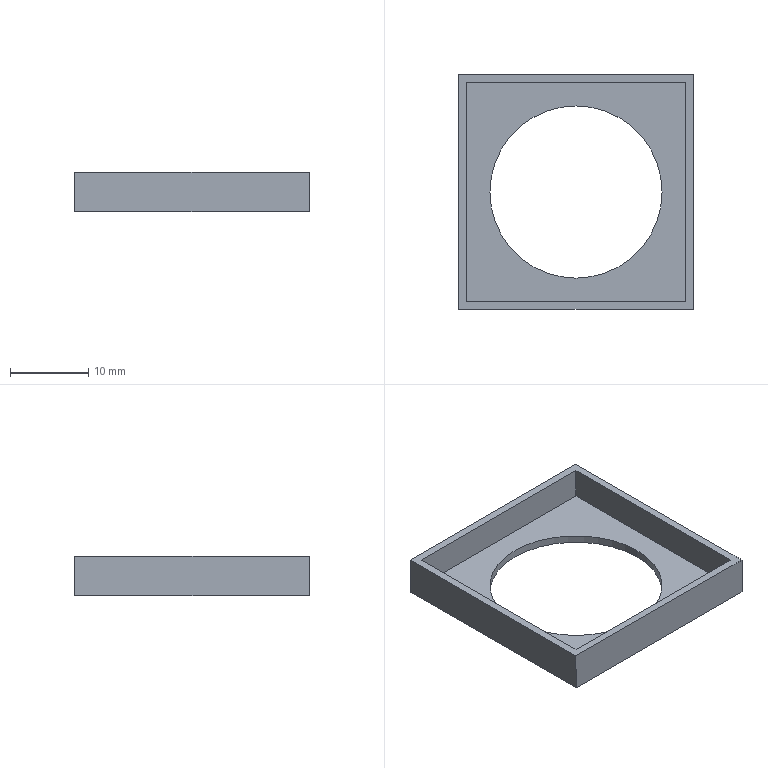Part | SolidWorks | features BossThin 1, Extrusion 1, ICE 1 | 1 solid | 13 faces | box 30 x 30 x 5 mm | volume 983.867 mm3 | plane 11 | cylinder 2 | commonest cylinder face diameters 22 x2
STEP:
#1=CARTESIAN_POINT('',(-11.,0.,0.));
#2=VERTEX_POINT('',#1);
#3=CARTESIAN_POINT('',(11.,0.,0.));
#4=VERTEX_POINT('',#3);
#5=CARTESIAN_POINT('',(0.,0.,0.));
#6=DIRECTION('',(0.,0.,1.));
#7=DIRECTION('',(1.,0.,0.));
#8=AXIS2_PLACEMENT_3D('',#5,#6,#7);
#9=CIRCLE('',#8,11.);
#10=EDGE_CURVE('',#2,#4,#9,.T.);
#11=ORIENTED_EDGE('',*,*,#10,.F.);
#12=CARTESIAN_POINT('',(-11.,0.,1.));
#13=VERTEX_POINT('',#12);
#14=CARTESIAN_POINT('',(-11.,0.,-4.));
#15=DIRECTION('',(0.,0.,1.));
#16=VECTOR('',#15,1000.);
#17=LINE('',#14,#16);
#18=EDGE_CURVE('',#2,#13,#17,.T.);
#19=ORIENTED_EDGE('',*,*,#18,.T.);
#20=CARTESIAN_POINT('',(11.,0.,1.));
#21=VERTEX_POINT('',#20);
#22=CARTESIAN_POINT('',(0.,0.,1.));
#23=DIRECTION('',(0.,0.,1.));
#24=DIRECTION('',(1.,0.,0.));
#25=AXIS2_PLACEMENT_3D('',#22,#23,#24);
#26=CIRCLE('',#25,11.);
#27=EDGE_CURVE('',#13,#21,#26,.T.);
#28=ORIENTED_EDGE('',*,*,#27,.T.);
#29=CARTESIAN_POINT('',(11.,0.,-4.));
#30=DIRECTION('',(0.,0.,1.));
#31=VECTOR('',#30,1000.);
#32=LINE('',#29,#31);
#33=EDGE_CURVE('',#4,#21,#32,.T.);
#34=ORIENTED_EDGE('',*,*,#33,.F.);
#35=EDGE_LOOP('',(#11,#19,#28,#34));
#36=FACE_OUTER_BOUND('',#35,.T.);
#37=CARTESIAN_POINT('',(0.,0.,-4.));
#38=DIRECTION('',(0.,0.,1.));
#39=DIRECTION('',(1.,0.,0.));
#40=AXIS2_PLACEMENT_3D('',#37,#38,#39);
#41=CYLINDRICAL_SURFACE('',#40,11.);
#42=ADVANCED_FACE('',(#36),#41,.F.);
#43=CARTESIAN_POINT('',(0.,0.,1.));
#44=DIRECTION('',(0.,0.,1.));
#45=DIRECTION('',(1.,0.,0.));
#46=AXIS2_PLACEMENT_3D('',#43,#44,#45);
#47=CIRCLE('',#46,11.);
#48=EDGE_CURVE('',#21,#13,#47,.T.);
#49=ORIENTED_EDGE('',*,*,#48,.F.);
#50=ORIENTED_EDGE('',*,*,#27,.F.);
#51=EDGE_LOOP('',(#49,#50));
#52=FACE_BOUND('',#51,.T.);
#53=CARTESIAN_POINT('',(14.,-14.,1.));
#54=VERTEX_POINT('',#53);
#55=CARTESIAN_POINT('',(14.,14.,1.));
#56=VERTEX_POINT('',#55);
#57=CARTESIAN_POINT('',(14.,14.,1.));
#58=DIRECTION('',(0.,1.,0.));
#59=VECTOR('',#58,1000.);
#60=LINE('',#57,#59);
#61=EDGE_CURVE('',#54,#56,#60,.T.);
#62=ORIENTED_EDGE('',*,*,#61,.T.);
#63=CARTESIAN_POINT('',(-14.,14.,1.));
#64=VERTEX_POINT('',#63);
#65=CARTESIAN_POINT('',(-14.,14.,1.));
#66=DIRECTION('',(-1.,0.,0.));
#67=VECTOR('',#66,1000.);
#68=LINE('',#65,#67);
#69=EDGE_CURVE('',#56,#64,#68,.T.);
#70=ORIENTED_EDGE('',*,*,#69,.T.);
#71=CARTESIAN_POINT('',(-14.,-14.,1.));
#72=VERTEX_POINT('',#71);
#73=CARTESIAN_POINT('',(-14.,14.,1.));
#74=DIRECTION('',(0.,-1.,0.));
#75=VECTOR('',#74,1000.);
#76=LINE('',#73,#75);
#77=EDGE_CURVE('',#64,#72,#76,.T.);
#78=ORIENTED_EDGE('',*,*,#77,.T.);
#79=CARTESIAN_POINT('',(-14.,-14.,1.));
#80=DIRECTION('',(1.,0.,0.));
#81=VECTOR('',#80,1000.);
#82=LINE('',#79,#81);
#83=EDGE_CURVE('',#72,#54,#82,.T.);
#84=ORIENTED_EDGE('',*,*,#83,.T.);
#85=EDGE_LOOP('',(#62,#70,#78,#84));
#86=FACE_OUTER_BOUND('',#85,.T.);
#87=CARTESIAN_POINT('',(0.,0.,1.));
#88=DIRECTION('',(0.,0.,1.));
#89=DIRECTION('',(1.,0.,0.));
#90=AXIS2_PLACEMENT_3D('',#87,#88,#89);
#91=PLANE('',#90);
#92=ADVANCED_FACE('',(#52,#86),#91,.T.);
#93=CARTESIAN_POINT('',(15.,-15.,5.));
#94=VERTEX_POINT('',#93);
#95=CARTESIAN_POINT('',(15.,15.,5.));
#96=VERTEX_POINT('',#95);
#97=CARTESIAN_POINT('',(15.,14.,5.));
#98=DIRECTION('',(0.,1.,0.));
#99=VECTOR('',#98,1000.);
#100=LINE('',#97,#99);
#101=EDGE_CURVE('',#94,#96,#100,.T.);
#102=ORIENTED_EDGE('',*,*,#101,.T.);
#103=CARTESIAN_POINT('',(-15.,15.,5.));
#104=VERTEX_POINT('',#103);
#105=CARTESIAN_POINT('',(-14.,15.,5.));
#106=DIRECTION('',(-1.,0.,0.));
#107=VECTOR('',#106,1000.);
#108=LINE('',#105,#107);
#109=EDGE_CURVE('',#96,#104,#108,.T.);
#110=ORIENTED_EDGE('',*,*,#109,.T.);
#111=CARTESIAN_POINT('',(-15.,-15.,5.));
#112=VERTEX_POINT('',#111);
#113=CARTESIAN_POINT('',(-15.,14.,5.));
#114=DIRECTION('',(0.,-1.,0.));
#115=VECTOR('',#114,1000.);
#116=LINE('',#113,#115);
#117=EDGE_CURVE('',#104,#112,#116,.T.);
#118=ORIENTED_EDGE('',*,*,#117,.T.);
#119=CARTESIAN_POINT('',(-14.,-15.,5.));
#120=DIRECTION('',(1.,0.,0.));
#121=VECTOR('',#120,1000.);
#122=LINE('',#119,#121);
#123=EDGE_CURVE('',#112,#94,#122,.T.);
#124=ORIENTED_EDGE('',*,*,#123,.T.);
#125=EDGE_LOOP('',(#102,#110,#118,#124));
#126=FACE_OUTER_BOUND('',#125,.T.);
#127=CARTESIAN_POINT('',(14.,14.,5.));
#128=VERTEX_POINT('',#127);
#129=CARTESIAN_POINT('',(-14.,14.,5.));
#130=VERTEX_POINT('',#129);
#131=CARTESIAN_POINT('',(-14.,14.,5.));
#132=DIRECTION('',(-1.,0.,0.));
#133=VECTOR('',#132,1000.);
#134=LINE('',#131,#133);
#135=EDGE_CURVE('',#128,#130,#134,.T.);
#136=ORIENTED_EDGE('',*,*,#135,.F.);
#137=CARTESIAN_POINT('',(14.,-14.,5.));
#138=VERTEX_POINT('',#137);
#139=CARTESIAN_POINT('',(14.,14.,5.));
#140=DIRECTION('',(0.,1.,0.));
#141=VECTOR('',#140,1000.);
#142=LINE('',#139,#141);
#143=EDGE_CURVE('',#138,#128,#142,.T.);
#144=ORIENTED_EDGE('',*,*,#143,.F.);
#145=CARTESIAN_POINT('',(-14.,-14.,5.));
#146=VERTEX_POINT('',#145);
#147=CARTESIAN_POINT('',(-14.,-14.,5.));
#148=DIRECTION('',(1.,0.,0.));
#149=VECTOR('',#148,1000.);
#150=LINE('',#147,#149);
#151=EDGE_CURVE('',#146,#138,#150,.T.);
#152=ORIENTED_EDGE('',*,*,#151,.F.);
#153=CARTESIAN_POINT('',(-14.,14.,5.));
#154=DIRECTION('',(0.,-1.,0.));
#155=VECTOR('',#154,1000.);
#156=LINE('',#153,#155);
#157=EDGE_CURVE('',#130,#146,#156,.T.);
#158=ORIENTED_EDGE('',*,*,#157,.F.);
#159=EDGE_LOOP('',(#136,#144,#152,#158));
#160=FACE_BOUND('',#159,.T.);
#161=CARTESIAN_POINT('',(0.,0.,5.));
#162=DIRECTION('',(0.,0.,1.));
#163=DIRECTION('',(1.,0.,0.));
#164=AXIS2_PLACEMENT_3D('',#161,#162,#163);
#165=PLANE('',#164);
#166=ADVANCED_FACE('',(#126,#160),#165,.T.);
#167=CARTESIAN_POINT('',(15.,-15.,0.));
#168=VERTEX_POINT('',#167);
#169=CARTESIAN_POINT('',(15.,15.,0.));
#170=VERTEX_POINT('',#169);
#171=CARTESIAN_POINT('',(15.,14.,0.));
#172=DIRECTION('',(0.,1.,0.));
#173=VECTOR('',#172,1000.);
#174=LINE('',#171,#173);
#175=EDGE_CURVE('',#168,#170,#174,.T.);
#176=ORIENTED_EDGE('',*,*,#175,.T.);
#177=CARTESIAN_POINT('',(15.,15.,5.));
#178=DIRECTION('',(0.,0.,-1.));
#179=VECTOR('',#178,1000.);
#180=LINE('',#177,#179);
#181=EDGE_CURVE('',#96,#170,#180,.T.);
#182=ORIENTED_EDGE('',*,*,#181,.F.);
#183=ORIENTED_EDGE('',*,*,#101,.F.);
#184=CARTESIAN_POINT('',(15.,-15.,5.));
#185=DIRECTION('',(0.,0.,-1.));
#186=VECTOR('',#185,1000.);
#187=LINE('',#184,#186);
#188=EDGE_CURVE('',#94,#168,#187,.T.);
#189=ORIENTED_EDGE('',*,*,#188,.T.);
#190=EDGE_LOOP('',(#176,#182,#183,#189));
#191=FACE_OUTER_BOUND('',#190,.T.);
#192=CARTESIAN_POINT('',(15.,14.,5.));
#193=DIRECTION('',(-1.,0.,0.));
#194=DIRECTION('',(0.,-1.,0.));
#195=AXIS2_PLACEMENT_3D('',#192,#193,#194);
#196=PLANE('',#195);
#197=ADVANCED_FACE('',(#191),#196,.F.);
#198=CARTESIAN_POINT('',(-15.,15.,0.));
#199=VERTEX_POINT('',#198);
#200=CARTESIAN_POINT('',(-14.,15.,0.));
#201=DIRECTION('',(-1.,0.,0.));
#202=VECTOR('',#201,1000.);
#203=LINE('',#200,#202);
#204=EDGE_CURVE('',#170,#199,#203,.T.);
#205=ORIENTED_EDGE('',*,*,#204,.T.);
#206=CARTESIAN_POINT('',(-15.,15.,5.));
#207=DIRECTION('',(0.,0.,-1.));
#208=VECTOR('',#207,1000.);
#209=LINE('',#206,#208);
#210=EDGE_CURVE('',#104,#199,#209,.T.);
#211=ORIENTED_EDGE('',*,*,#210,.F.);
#212=ORIENTED_EDGE('',*,*,#109,.F.);
#213=ORIENTED_EDGE('',*,*,#181,.T.);
#214=EDGE_LOOP('',(#205,#211,#212,#213));
#215=FACE_OUTER_BOUND('',#214,.T.);
#216=CARTESIAN_POINT('',(-14.,15.,5.));
#217=DIRECTION('',(0.,-1.,0.));
#218=DIRECTION('',(0.,0.,-1.));
#219=AXIS2_PLACEMENT_3D('',#216,#217,#218);
#220=PLANE('',#219);
#221=ADVANCED_FACE('',(#215),#220,.F.);
#222=CARTESIAN_POINT('',(-15.,-15.,0.));
#223=VERTEX_POINT('',#222);
#224=CARTESIAN_POINT('',(-15.,14.,0.));
#225=DIRECTION('',(0.,-1.,0.));
#226=VECTOR('',#225,1000.);
#227=LINE('',#224,#226);
#228=EDGE_CURVE('',#199,#223,#227,.T.);
#229=ORIENTED_EDGE('',*,*,#228,.T.);
#230=CARTESIAN_POINT('',(-15.,-15.,5.));
#231=DIRECTION('',(0.,0.,-1.));
#232=VECTOR('',#231,1000.);
#233=LINE('',#230,#232);
#234=EDGE_CURVE('',#112,#223,#233,.T.);
#235=ORIENTED_EDGE('',*,*,#234,.F.);
#236=ORIENTED_EDGE('',*,*,#117,.F.);
#237=ORIENTED_EDGE('',*,*,#210,.T.);
#238=EDGE_LOOP('',(#229,#235,#236,#237));
#239=FACE_OUTER_BOUND('',#238,.T.);
#240=CARTESIAN_POINT('',(-15.,14.,5.));
#241=DIRECTION('',(1.,0.,0.));
#242=DIRECTION('',(0.,1.,0.));
#243=AXIS2_PLACEMENT_3D('',#240,#241,#242);
#244=PLANE('',#243);
#245=ADVANCED_FACE('',(#239),#244,.F.);
#246=CARTESIAN_POINT('',(-14.,-15.,0.));
#247=DIRECTION('',(1.,0.,0.));
#248=VECTOR('',#247,1000.);
#249=LINE('',#246,#248);
#250=EDGE_CURVE('',#223,#168,#249,.T.);
#251=ORIENTED_EDGE('',*,*,#250,.T.);
#252=ORIENTED_EDGE('',*,*,#188,.F.);
#253=ORIENTED_EDGE('',*,*,#123,.F.);
#254=ORIENTED_EDGE('',*,*,#234,.T.);
#255=EDGE_LOOP('',(#251,#252,#253,#254));
#256=FACE_OUTER_BOUND('',#255,.T.);
#257=CARTESIAN_POINT('',(-14.,-15.,5.));
#258=DIRECTION('',(0.,1.,0.));
#259=DIRECTION('',(0.,0.,1.));
#260=AXIS2_PLACEMENT_3D('',#257,#258,#259);
#261=PLANE('',#260);
#262=ADVANCED_FACE('',(#256),#261,.F.);
#263=CARTESIAN_POINT('',(14.,14.,5.));
#264=DIRECTION('',(0.,0.,-1.));
#265=VECTOR('',#264,1000.);
#266=LINE('',#263,#265);
#267=EDGE_CURVE('',#128,#56,#266,.T.);
#268=ORIENTED_EDGE('',*,*,#267,.T.);
#269=ORIENTED_EDGE('',*,*,#61,.F.);
#270=CARTESIAN_POINT('',(14.,-14.,5.));
#271=DIRECTION('',(0.,0.,-1.));
#272=VECTOR('',#271,1000.);
#273=LINE('',#270,#272);
#274=EDGE_CURVE('',#138,#54,#273,.T.);
#275=ORIENTED_EDGE('',*,*,#274,.F.);
#276=ORIENTED_EDGE('',*,*,#143,.T.);
#277=EDGE_LOOP('',(#268,#269,#275,#276));
#278=FACE_OUTER_BOUND('',#277,.T.);
#279=CARTESIAN_POINT('',(14.,14.,5.));
#280=DIRECTION('',(-1.,0.,0.));
#281=DIRECTION('',(0.,-1.,0.));
#282=AXIS2_PLACEMENT_3D('',#279,#280,#281);
#283=PLANE('',#282);
#284=ADVANCED_FACE('',(#278),#283,.T.);
#285=CARTESIAN_POINT('',(-14.,14.,5.));
#286=DIRECTION('',(0.,0.,-1.));
#287=VECTOR('',#286,1000.);
#288=LINE('',#285,#287);
#289=EDGE_CURVE('',#130,#64,#288,.T.);
#290=ORIENTED_EDGE('',*,*,#289,.T.);
#291=ORIENTED_EDGE('',*,*,#69,.F.);
#292=ORIENTED_EDGE('',*,*,#267,.F.);
#293=ORIENTED_EDGE('',*,*,#135,.T.);
#294=EDGE_LOOP('',(#290,#291,#292,#293));
#295=FACE_OUTER_BOUND('',#294,.T.);
#296=CARTESIAN_POINT('',(-14.,14.,5.));
#297=DIRECTION('',(0.,-1.,0.));
#298=DIRECTION('',(0.,0.,-1.));
#299=AXIS2_PLACEMENT_3D('',#296,#297,#298);
#300=PLANE('',#299);
#301=ADVANCED_FACE('',(#295),#300,.T.);
#302=CARTESIAN_POINT('',(-14.,-14.,5.));
#303=DIRECTION('',(0.,0.,-1.));
#304=VECTOR('',#303,1000.);
#305=LINE('',#302,#304);
#306=EDGE_CURVE('',#146,#72,#305,.T.);
#307=ORIENTED_EDGE('',*,*,#306,.T.);
#308=ORIENTED_EDGE('',*,*,#77,.F.);
#309=ORIENTED_EDGE('',*,*,#289,.F.);
#310=ORIENTED_EDGE('',*,*,#157,.T.);
#311=EDGE_LOOP('',(#307,#308,#309,#310));
#312=FACE_OUTER_BOUND('',#311,.T.);
#313=CARTESIAN_POINT('',(-14.,14.,5.));
#314=DIRECTION('',(1.,0.,0.));
#315=DIRECTION('',(0.,1.,0.));
#316=AXIS2_PLACEMENT_3D('',#313,#314,#315);
#317=PLANE('',#316);
#318=ADVANCED_FACE('',(#312),#317,.T.);
#319=ORIENTED_EDGE('',*,*,#274,.T.);
#320=ORIENTED_EDGE('',*,*,#83,.F.);
#321=ORIENTED_EDGE('',*,*,#306,.F.);
#322=ORIENTED_EDGE('',*,*,#151,.T.);
#323=EDGE_LOOP('',(#319,#320,#321,#322));
#324=FACE_OUTER_BOUND('',#323,.T.);
#325=CARTESIAN_POINT('',(-14.,-14.,5.));
#326=DIRECTION('',(0.,1.,0.));
#327=DIRECTION('',(0.,0.,1.));
#328=AXIS2_PLACEMENT_3D('',#325,#326,#327);
#329=PLANE('',#328);
#330=ADVANCED_FACE('',(#324),#329,.T.);
#331=CARTESIAN_POINT('',(0.,0.,0.));
#332=DIRECTION('',(0.,0.,1.));
#333=DIRECTION('',(1.,0.,0.));
#334=AXIS2_PLACEMENT_3D('',#331,#332,#333);
#335=CIRCLE('',#334,11.);
#336=EDGE_CURVE('',#4,#2,#335,.T.);
#337=ORIENTED_EDGE('',*,*,#336,.T.);
#338=ORIENTED_EDGE('',*,*,#10,.T.);
#339=EDGE_LOOP('',(#337,#338));
#340=FACE_BOUND('',#339,.T.);
#341=ORIENTED_EDGE('',*,*,#175,.F.);
#342=ORIENTED_EDGE('',*,*,#250,.F.);
#343=ORIENTED_EDGE('',*,*,#228,.F.);
#344=ORIENTED_EDGE('',*,*,#204,.F.);
#345=EDGE_LOOP('',(#341,#342,#343,#344));
#346=FACE_OUTER_BOUND('',#345,.T.);
#347=CARTESIAN_POINT('',(0.,0.,0.));
#348=DIRECTION('',(0.,0.,1.));
#349=DIRECTION('',(1.,0.,0.));
#350=AXIS2_PLACEMENT_3D('',#347,#348,#349);
#351=PLANE('',#350);
#352=ADVANCED_FACE('',(#340,#346),#351,.F.);
#353=ORIENTED_EDGE('',*,*,#18,.F.);
#354=ORIENTED_EDGE('',*,*,#336,.F.);
#355=ORIENTED_EDGE('',*,*,#33,.T.);
#356=ORIENTED_EDGE('',*,*,#48,.T.);
#357=EDGE_LOOP('',(#353,#354,#355,#356));
#358=FACE_OUTER_BOUND('',#357,.T.);
#359=CARTESIAN_POINT('',(0.,0.,-4.));
#360=DIRECTION('',(0.,0.,1.));
#361=DIRECTION('',(1.,0.,0.));
#362=AXIS2_PLACEMENT_3D('',#359,#360,#361);
#363=CYLINDRICAL_SURFACE('',#362,11.);
#364=ADVANCED_FACE('',(#358),#363,.F.);
#365=CLOSED_SHELL('',(#42,#92,#166,#197,#221,#245,#262,#284,#301,#318,#330,#352,#364));
#366=MANIFOLD_SOLID_BREP('',#365);
#367=CARTESIAN_POINT('',(0.,0.,0.));
#368=DIRECTION('',(0.,0.,1.));
#369=DIRECTION('',(1.,0.,0.));
#370=AXIS2_PLACEMENT_3D('',#367,#368,#369);
#371=(LENGTH_UNIT()NAMED_UNIT(*)SI_UNIT(.MILLI.,.METRE.));
#372=UNCERTAINTY_MEASURE_WITH_UNIT(LENGTH_MEASURE(0.00001),#371,'','');
#373=(NAMED_UNIT(*)PLANE_ANGLE_UNIT()SI_UNIT($,.RADIAN.));
#374=(NAMED_UNIT(*)SI_UNIT($,.STERADIAN.)SOLID_ANGLE_UNIT());
#375=(GEOMETRIC_REPRESENTATION_CONTEXT(3)GLOBAL_UNCERTAINTY_ASSIGNED_CONTEXT((#372))GLOBAL_UNIT_ASSIGNED_CONTEXT((#371,#373,#374))REPRESENTATION_CONTEXT('',''));
#376=ADVANCED_BREP_SHAPE_REPRESENTATION('',(#366,#370),#375);